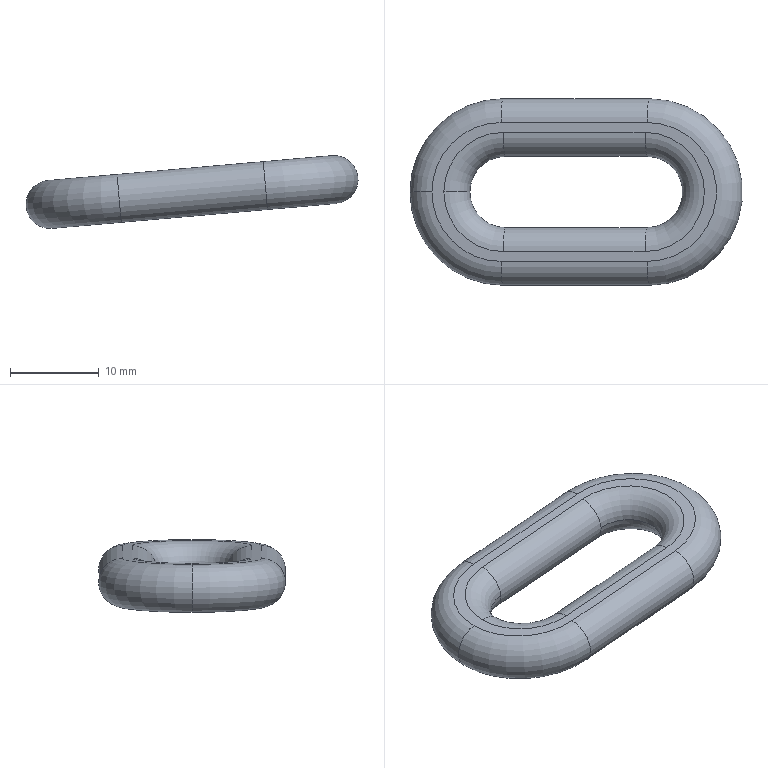Part | STEP file | 871-10_1m (label)-Part-1 | 1 solid | 15 faces | box 37.378 x 21 x 8.198 mm | volume 2290 mm3 | torus 9 | cylinder 4 | plane 2 | commonest cylinder face diameters 5.4 x4
STEP:
#1=CARTESIAN_POINT('',(0.,0.,0.));
#2=DIRECTION('',(0.,0.,1.));
#3=DIRECTION('',(1.,0.,0.));
#4=AXIS2_PLACEMENT_3D('',#1,#2,#3);
#5=CARTESIAN_POINT('',(26.368,17.2,8.756));
#6=VERTEX_POINT('',#5);
#7=CARTESIAN_POINT('',(26.603,14.5,6.066));
#8=VERTEX_POINT('',#7);
#9=CARTESIAN_POINT('',(26.603,17.2,6.066));
#10=DIRECTION('',(0.9962,0.,0.08716));
#11=DIRECTION('',(0.08716,0.,-0.9962));
#12=AXIS2_PLACEMENT_3D('',#9,#10,#11);
#13=CIRCLE('',#12,2.7);
#14=CARTESIAN_POINT('',(26.603,10.5,6.066));
#15=DIRECTION('',(0.08716,0.,-0.9962));
#16=DIRECTION('',(-0.9962,0.,-0.08716));
#17=AXIS2_PLACEMENT_3D('',#14,#15,#16);
#18=TOROIDAL_SURFACE('',#17,6.7,2.7);
#19=CARTESIAN_POINT('',(1.571,7.854));
#20=DIRECTION('',(0.,-1.));
#21=VECTOR('',#20,1.);
#22=LINE('',#19,#21);
#23=(GEOMETRIC_REPRESENTATION_CONTEXT(2)PARAMETRIC_REPRESENTATION_CONTEXT()REPRESENTATION_CONTEXT('',''));
#24=DEFINITIONAL_REPRESENTATION('',(#22),#23);
#25=PCURVE('',#18,#24);
#26=CARTESIAN_POINT('',(18.633,17.2,5.369));
#27=DIRECTION('',(0.9962,0.,0.08716));
#28=DIRECTION('',(0.08716,0.,-0.9962));
#29=AXIS2_PLACEMENT_3D('',#26,#27,#28);
#30=CYLINDRICAL_SURFACE('',#29,2.7);
#31=CARTESIAN_POINT('',(0.,8.));
#32=DIRECTION('',(1.,0.));
#33=VECTOR('',#32,1.);
#34=LINE('',#31,#33);
#35=(GEOMETRIC_REPRESENTATION_CONTEXT(2)PARAMETRIC_REPRESENTATION_CONTEXT()REPRESENTATION_CONTEXT('',''));
#36=DEFINITIONAL_REPRESENTATION('',(#34),#35);
#37=PCURVE('',#30,#36);
#38=SURFACE_CURVE('',#13,(#25,#37),.PCURVE_S1.);
#39=EDGE_CURVE('',#6,#8,#38,.T.);
#40=ORIENTED_EDGE('',*,*,#39,.T.);
#41=CARTESIAN_POINT('',(26.603,6.5,6.066));
#42=VERTEX_POINT('',#41);
#43=CARTESIAN_POINT('',(26.603,10.5,6.066));
#44=DIRECTION('',(0.08716,0.,-0.9962));
#45=DIRECTION('',(-0.9962,0.,-0.08716));
#46=AXIS2_PLACEMENT_3D('',#43,#44,#45);
#47=CIRCLE('',#46,4.);
#48=CARTESIAN_POINT('',(0.,3.142));
#49=DIRECTION('',(1.,0.));
#50=VECTOR('',#49,1.);
#51=LINE('',#48,#50);
#52=(GEOMETRIC_REPRESENTATION_CONTEXT(2)PARAMETRIC_REPRESENTATION_CONTEXT()REPRESENTATION_CONTEXT('',''));
#53=DEFINITIONAL_REPRESENTATION('',(#51),#52);
#54=PCURVE('',#18,#53);
#55=CARTESIAN_POINT('',(26.603,10.5,6.066));
#56=DIRECTION('',(0.08716,0.,-0.9962));
#57=DIRECTION('',(-0.9962,0.,-0.08716));
#58=AXIS2_PLACEMENT_3D('',#55,#56,#57);
#59=TOROIDAL_SURFACE('',#58,6.7,2.7);
#60=CARTESIAN_POINT('',(0.,3.142));
#61=DIRECTION('',(1.,0.));
#62=VECTOR('',#61,1.);
#63=LINE('',#60,#62);
#64=(GEOMETRIC_REPRESENTATION_CONTEXT(2)PARAMETRIC_REPRESENTATION_CONTEXT()REPRESENTATION_CONTEXT('',''));
#65=DEFINITIONAL_REPRESENTATION('',(#63),#64);
#66=PCURVE('',#59,#65);
#67=SURFACE_CURVE('',#47,(#54,#66),.PCURVE_S1.);
#68=EDGE_CURVE('',#8,#42,#67,.T.);
#69=ORIENTED_EDGE('',*,*,#68,.T.);
#70=CARTESIAN_POINT('',(26.368,3.8,8.756));
#71=VERTEX_POINT('',#70);
#72=CARTESIAN_POINT('',(26.603,3.8,6.066));
#73=DIRECTION('',(-0.9962,0.,-0.08716));
#74=DIRECTION('',(-0.08716,0.,0.9962));
#75=AXIS2_PLACEMENT_3D('',#72,#73,#74);
#76=CIRCLE('',#75,2.7);
#77=CARTESIAN_POINT('',(4.712,4.712));
#78=DIRECTION('',(0.,-1.));
#79=VECTOR('',#78,1.);
#80=LINE('',#77,#79);
#81=(GEOMETRIC_REPRESENTATION_CONTEXT(2)PARAMETRIC_REPRESENTATION_CONTEXT()REPRESENTATION_CONTEXT('',''));
#82=DEFINITIONAL_REPRESENTATION('',(#80),#81);
#83=PCURVE('',#18,#82);
#84=CARTESIAN_POINT('',(18.633,3.8,5.369));
#85=DIRECTION('',(-0.9962,0.,-0.08716));
#86=DIRECTION('',(-0.08716,0.,0.9962));
#87=AXIS2_PLACEMENT_3D('',#84,#85,#86);
#88=CYLINDRICAL_SURFACE('',#87,2.7);
#89=CARTESIAN_POINT('',(0.,-8.));
#90=DIRECTION('',(1.,0.));
#91=VECTOR('',#90,1.);
#92=LINE('',#89,#91);
#93=(GEOMETRIC_REPRESENTATION_CONTEXT(2)PARAMETRIC_REPRESENTATION_CONTEXT()REPRESENTATION_CONTEXT('',''));
#94=DEFINITIONAL_REPRESENTATION('',(#92),#93);
#95=PCURVE('',#88,#94);
#96=SURFACE_CURVE('',#76,(#83,#95),.PCURVE_S1.);
#97=EDGE_CURVE('',#71,#42,#96,.T.);
#98=ORIENTED_EDGE('',*,*,#97,.F.);
#99=CARTESIAN_POINT('',(26.368,10.5,8.756));
#100=DIRECTION('',(0.08716,0.,-0.9962));
#101=DIRECTION('',(0.9962,0.,0.08716));
#102=AXIS2_PLACEMENT_3D('',#99,#100,#101);
#103=CIRCLE('',#102,6.7);
#104=CARTESIAN_POINT('',(-3.142,4.712));
#105=DIRECTION('',(1.,0.));
#106=VECTOR('',#105,1.);
#107=LINE('',#104,#106);
#108=(GEOMETRIC_REPRESENTATION_CONTEXT(2)PARAMETRIC_REPRESENTATION_CONTEXT()REPRESENTATION_CONTEXT('',''));
#109=DEFINITIONAL_REPRESENTATION('',(#107),#108);
#110=PCURVE('',#18,#109);
#111=CARTESIAN_POINT('',(18.398,10.5,8.059));
#112=DIRECTION('',(-0.08716,0.,0.9962));
#113=DIRECTION('',(0.9962,0.,0.08716));
#114=AXIS2_PLACEMENT_3D('',#111,#112,#113);
#115=PLANE('',#114);
#116=CARTESIAN_POINT('',(14.7,0.));
#117=CARTESIAN_POINT('',(14.7,-11.605));
#118=CARTESIAN_POINT('',(4.65,-5.802));
#119=CARTESIAN_POINT('',(-5.4,0.));
#120=CARTESIAN_POINT('',(4.65,5.802));
#121=CARTESIAN_POINT('',(14.7,11.605));
#122=CARTESIAN_POINT('',(14.7,0.));
#123=(BOUNDED_CURVE()B_SPLINE_CURVE(2,(#116,#117,#118,#119,#120,#121,#122),.UNSPECIFIED.,.T.,.F.)B_SPLINE_CURVE_WITH_KNOTS((1,2,2,2,2,1),(-2.094,0.,2.094,4.189,6.283,8.378),.UNSPECIFIED.)CURVE()GEOMETRIC_REPRESENTATION_ITEM()RATIONAL_B_SPLINE_CURVE((1.,0.5,1.,0.5,1.,0.5,1.))REPRESENTATION_ITEM(''));
#124=(GEOMETRIC_REPRESENTATION_CONTEXT(2)PARAMETRIC_REPRESENTATION_CONTEXT()REPRESENTATION_CONTEXT('',''));
#125=DEFINITIONAL_REPRESENTATION('',(#123),#124);
#126=PCURVE('',#115,#125);
#127=SURFACE_CURVE('',#103,(#110,#126),.PCURVE_S1.);
#128=EDGE_CURVE('',#6,#71,#127,.T.);
#129=ORIENTED_EDGE('',*,*,#128,.F.);
#130=EDGE_LOOP('',(#40,#69,#98,#129));
#131=FACE_BOUND('',#130,.T.);
#132=ADVANCED_FACE('',(#131),#18,.T.);
#133=CARTESIAN_POINT('',(6.679,10.5,4.323));
#134=VERTEX_POINT('',#133);
#135=CARTESIAN_POINT('',(3.754,10.5,6.778));
#136=VERTEX_POINT('',#135);
#137=CARTESIAN_POINT('',(3.989,10.5,4.088));
#138=DIRECTION('',(0.,-1.,0.));
#139=DIRECTION('',(1.,0.,0.));
#140=AXIS2_PLACEMENT_3D('',#137,#138,#139);
#141=CIRCLE('',#140,2.7);
#142=CARTESIAN_POINT('',(10.664,10.5,4.672));
#143=DIRECTION('',(0.08716,0.,-0.9962));
#144=DIRECTION('',(-0.9962,0.,-0.08716));
#145=AXIS2_PLACEMENT_3D('',#142,#143,#144);
#146=TOROIDAL_SURFACE('',#145,6.7,2.7);
#147=CARTESIAN_POINT('',(0.,3.054));
#148=DIRECTION('',(0.,1.));
#149=VECTOR('',#148,1.);
#150=LINE('',#147,#149);
#151=(GEOMETRIC_REPRESENTATION_CONTEXT(2)PARAMETRIC_REPRESENTATION_CONTEXT()REPRESENTATION_CONTEXT('',''));
#152=DEFINITIONAL_REPRESENTATION('',(#150),#151);
#153=PCURVE('',#146,#152);
#154=CARTESIAN_POINT('',(10.664,10.5,4.672));
#155=DIRECTION('',(0.08716,0.,-0.9962));
#156=DIRECTION('',(-0.9962,0.,-0.08716));
#157=AXIS2_PLACEMENT_3D('',#154,#155,#156);
#158=TOROIDAL_SURFACE('',#157,6.7,2.7);
#159=CARTESIAN_POINT('',(6.283,3.054));
#160=DIRECTION('',(0.,1.));
#161=VECTOR('',#160,1.);
#162=LINE('',#159,#161);
#163=(GEOMETRIC_REPRESENTATION_CONTEXT(2)PARAMETRIC_REPRESENTATION_CONTEXT()REPRESENTATION_CONTEXT('',''));
#164=DEFINITIONAL_REPRESENTATION('',(#162),#163);
#165=PCURVE('',#158,#164);
#166=SURFACE_CURVE('',#141,(#153,#165),.PCURVE_S1.);
#167=EDGE_CURVE('',#134,#136,#166,.T.);
#168=ORIENTED_EDGE('',*,*,#167,.F.);
#169=CARTESIAN_POINT('',(10.664,14.5,4.672));
#170=VERTEX_POINT('',#169);
#171=CARTESIAN_POINT('',(10.664,10.5,4.672));
#172=DIRECTION('',(0.08716,0.,-0.9962));
#173=DIRECTION('',(-0.9962,0.,-0.08716));
#174=AXIS2_PLACEMENT_3D('',#171,#172,#173);
#175=CIRCLE('',#174,4.);
#176=CARTESIAN_POINT('',(0.,3.142));
#177=DIRECTION('',(1.,0.));
#178=VECTOR('',#177,1.);
#179=LINE('',#176,#178);
#180=(GEOMETRIC_REPRESENTATION_CONTEXT(2)PARAMETRIC_REPRESENTATION_CONTEXT()REPRESENTATION_CONTEXT('',''));
#181=DEFINITIONAL_REPRESENTATION('',(#179),#180);
#182=PCURVE('',#146,#181);
#183=CARTESIAN_POINT('',(10.664,10.5,4.672));
#184=DIRECTION('',(0.08716,0.,-0.9962));
#185=DIRECTION('',(-0.9962,0.,-0.08716));
#186=AXIS2_PLACEMENT_3D('',#183,#184,#185);
#187=TOROIDAL_SURFACE('',#186,6.7,2.7);
#188=CARTESIAN_POINT('',(0.,3.142));
#189=DIRECTION('',(1.,0.));
#190=VECTOR('',#189,1.);
#191=LINE('',#188,#190);
#192=(GEOMETRIC_REPRESENTATION_CONTEXT(2)PARAMETRIC_REPRESENTATION_CONTEXT()REPRESENTATION_CONTEXT('',''));
#193=DEFINITIONAL_REPRESENTATION('',(#191),#192);
#194=PCURVE('',#187,#193);
#195=SURFACE_CURVE('',#175,(#182,#194),.PCURVE_S1.);
#196=EDGE_CURVE('',#134,#170,#195,.T.);
#197=ORIENTED_EDGE('',*,*,#196,.T.);
#198=CARTESIAN_POINT('',(10.429,17.2,7.362));
#199=VERTEX_POINT('',#198);
#200=CARTESIAN_POINT('',(10.664,17.2,4.672));
#201=DIRECTION('',(-0.9962,0.,-0.08716));
#202=DIRECTION('',(-0.08716,0.,0.9962));
#203=AXIS2_PLACEMENT_3D('',#200,#201,#202);
#204=CIRCLE('',#203,2.7);
#205=CARTESIAN_POINT('',(1.571,-1.571));
#206=DIRECTION('',(0.,1.));
#207=VECTOR('',#206,1.);
#208=LINE('',#205,#207);
#209=(GEOMETRIC_REPRESENTATION_CONTEXT(2)PARAMETRIC_REPRESENTATION_CONTEXT()REPRESENTATION_CONTEXT('',''));
#210=DEFINITIONAL_REPRESENTATION('',(#208),#209);
#211=PCURVE('',#146,#210);
#212=CARTESIAN_POINT('',(9.425,-8.));
#213=DIRECTION('',(-1.,0.));
#214=VECTOR('',#213,1.);
#215=LINE('',#212,#214);
#216=(GEOMETRIC_REPRESENTATION_CONTEXT(2)PARAMETRIC_REPRESENTATION_CONTEXT()REPRESENTATION_CONTEXT('',''));
#217=DEFINITIONAL_REPRESENTATION('',(#215),#216);
#218=PCURVE('',#30,#217);
#219=SURFACE_CURVE('',#204,(#211,#218),.PCURVE_S1.);
#220=EDGE_CURVE('',#170,#199,#219,.T.);
#221=ORIENTED_EDGE('',*,*,#220,.T.);
#222=CARTESIAN_POINT('',(10.429,10.5,7.362));
#223=DIRECTION('',(0.08716,0.,-0.9962));
#224=DIRECTION('',(0.9962,0.,0.08716));
#225=AXIS2_PLACEMENT_3D('',#222,#223,#224);
#226=CIRCLE('',#225,6.7);
#227=CARTESIAN_POINT('',(-3.142,4.712));
#228=DIRECTION('',(1.,0.));
#229=VECTOR('',#228,1.);
#230=LINE('',#227,#229);
#231=(GEOMETRIC_REPRESENTATION_CONTEXT(2)PARAMETRIC_REPRESENTATION_CONTEXT()REPRESENTATION_CONTEXT('',''));
#232=DEFINITIONAL_REPRESENTATION('',(#230),#231);
#233=PCURVE('',#146,#232);
#234=CARTESIAN_POINT('',(-1.3,0.));
#235=CARTESIAN_POINT('',(-1.3,-11.605));
#236=CARTESIAN_POINT('',(-11.35,-5.802));
#237=CARTESIAN_POINT('',(-21.4,0.));
#238=CARTESIAN_POINT('',(-11.35,5.802));
#239=CARTESIAN_POINT('',(-1.3,11.605));
#240=CARTESIAN_POINT('',(-1.3,0.));
#241=(BOUNDED_CURVE()B_SPLINE_CURVE(2,(#234,#235,#236,#237,#238,#239,#240),.UNSPECIFIED.,.T.,.F.)B_SPLINE_CURVE_WITH_KNOTS((1,2,2,2,2,1),(-2.094,0.,2.094,4.189,6.283,8.378),.UNSPECIFIED.)CURVE()GEOMETRIC_REPRESENTATION_ITEM()RATIONAL_B_SPLINE_CURVE((1.,0.5,1.,0.5,1.,0.5,1.))REPRESENTATION_ITEM(''));
#242=(GEOMETRIC_REPRESENTATION_CONTEXT(2)PARAMETRIC_REPRESENTATION_CONTEXT()REPRESENTATION_CONTEXT('',''));
#243=DEFINITIONAL_REPRESENTATION('',(#241),#242);
#244=PCURVE('',#115,#243);
#245=SURFACE_CURVE('',#226,(#233,#244),.PCURVE_S1.);
#246=EDGE_CURVE('',#136,#199,#245,.T.);
#247=ORIENTED_EDGE('',*,*,#246,.F.);
#248=EDGE_LOOP('',(#168,#197,#221,#247));
#249=FACE_BOUND('',#248,.T.);
#250=ADVANCED_FACE('',(#249),#146,.T.);
#251=CARTESIAN_POINT('',(10.664,6.5,4.672));
#252=VERTEX_POINT('',#251);
#253=CARTESIAN_POINT('',(10.429,3.8,7.362));
#254=VERTEX_POINT('',#253);
#255=CARTESIAN_POINT('',(10.664,3.8,4.672));
#256=DIRECTION('',(0.9962,0.,0.08716));
#257=DIRECTION('',(0.08716,0.,-0.9962));
#258=AXIS2_PLACEMENT_3D('',#255,#256,#257);
#259=CIRCLE('',#258,2.7);
#260=CARTESIAN_POINT('',(4.712,1.571));
#261=DIRECTION('',(0.,1.));
#262=VECTOR('',#261,1.);
#263=LINE('',#260,#262);
#264=(GEOMETRIC_REPRESENTATION_CONTEXT(2)PARAMETRIC_REPRESENTATION_CONTEXT()REPRESENTATION_CONTEXT('',''));
#265=DEFINITIONAL_REPRESENTATION('',(#263),#264);
#266=PCURVE('',#158,#265);
#267=CARTESIAN_POINT('',(3.142,8.));
#268=DIRECTION('',(-1.,0.));
#269=VECTOR('',#268,1.);
#270=LINE('',#267,#269);
#271=(GEOMETRIC_REPRESENTATION_CONTEXT(2)PARAMETRIC_REPRESENTATION_CONTEXT()REPRESENTATION_CONTEXT('',''));
#272=DEFINITIONAL_REPRESENTATION('',(#270),#271);
#273=PCURVE('',#88,#272);
#274=SURFACE_CURVE('',#259,(#266,#273),.PCURVE_S1.);
#275=EDGE_CURVE('',#252,#254,#274,.T.);
#276=ORIENTED_EDGE('',*,*,#275,.F.);
#277=CARTESIAN_POINT('',(10.664,10.5,4.672));
#278=DIRECTION('',(0.08716,0.,-0.9962));
#279=DIRECTION('',(-0.9962,0.,-0.08716));
#280=AXIS2_PLACEMENT_3D('',#277,#278,#279);
#281=CIRCLE('',#280,4.);
#282=CARTESIAN_POINT('',(0.,3.142));
#283=DIRECTION('',(1.,0.));
#284=VECTOR('',#283,1.);
#285=LINE('',#282,#284);
#286=(GEOMETRIC_REPRESENTATION_CONTEXT(2)PARAMETRIC_REPRESENTATION_CONTEXT()REPRESENTATION_CONTEXT('',''));
#287=DEFINITIONAL_REPRESENTATION('',(#285),#286);
#288=PCURVE('',#158,#287);
#289=CARTESIAN_POINT('',(10.664,10.5,4.672));
#290=DIRECTION('',(0.08716,0.,-0.9962));
#291=DIRECTION('',(-0.9962,0.,-0.08716));
#292=AXIS2_PLACEMENT_3D('',#289,#290,#291);
#293=TOROIDAL_SURFACE('',#292,6.7,2.7);
#294=CARTESIAN_POINT('',(0.,3.142));
#295=DIRECTION('',(1.,0.));
#296=VECTOR('',#295,1.);
#297=LINE('',#294,#296);
#298=(GEOMETRIC_REPRESENTATION_CONTEXT(2)PARAMETRIC_REPRESENTATION_CONTEXT()REPRESENTATION_CONTEXT('',''));
#299=DEFINITIONAL_REPRESENTATION('',(#297),#298);
#300=PCURVE('',#293,#299);
#301=SURFACE_CURVE('',#281,(#288,#300),.PCURVE_S1.);
#302=EDGE_CURVE('',#252,#134,#301,.T.);
#303=ORIENTED_EDGE('',*,*,#302,.T.);
#304=ORIENTED_EDGE('',*,*,#167,.T.);
#305=CARTESIAN_POINT('',(10.429,10.5,7.362));
#306=DIRECTION('',(0.08716,0.,-0.9962));
#307=DIRECTION('',(0.9962,0.,0.08716));
#308=AXIS2_PLACEMENT_3D('',#305,#306,#307);
#309=CIRCLE('',#308,6.7);
#310=CARTESIAN_POINT('',(3.142,4.712));
#311=DIRECTION('',(1.,0.));
#312=VECTOR('',#311,1.);
#313=LINE('',#310,#312);
#314=(GEOMETRIC_REPRESENTATION_CONTEXT(2)PARAMETRIC_REPRESENTATION_CONTEXT()REPRESENTATION_CONTEXT('',''));
#315=DEFINITIONAL_REPRESENTATION('',(#313),#314);
#316=PCURVE('',#158,#315);
#317=CARTESIAN_POINT('',(-1.3,0.));
#318=CARTESIAN_POINT('',(-1.3,-11.605));
#319=CARTESIAN_POINT('',(-11.35,-5.802));
#320=CARTESIAN_POINT('',(-21.4,0.));
#321=CARTESIAN_POINT('',(-11.35,5.802));
#322=CARTESIAN_POINT('',(-1.3,11.605));
#323=CARTESIAN_POINT('',(-1.3,0.));
#324=(BOUNDED_CURVE()B_SPLINE_CURVE(2,(#317,#318,#319,#320,#321,#322,#323),.UNSPECIFIED.,.T.,.F.)B_SPLINE_CURVE_WITH_KNOTS((1,2,2,2,2,1),(-2.094,0.,2.094,4.189,6.283,8.378),.UNSPECIFIED.)CURVE()GEOMETRIC_REPRESENTATION_ITEM()RATIONAL_B_SPLINE_CURVE((1.,0.5,1.,0.5,1.,0.5,1.))REPRESENTATION_ITEM(''));
#325=(GEOMETRIC_REPRESENTATION_CONTEXT(2)PARAMETRIC_REPRESENTATION_CONTEXT()REPRESENTATION_CONTEXT('',''));
#326=DEFINITIONAL_REPRESENTATION('',(#324),#325);
#327=PCURVE('',#115,#326);
#328=SURFACE_CURVE('',#309,(#316,#327),.PCURVE_S1.);
#329=EDGE_CURVE('',#254,#136,#328,.T.);
#330=ORIENTED_EDGE('',*,*,#329,.F.);
#331=EDGE_LOOP('',(#276,#303,#304,#330));
#332=FACE_BOUND('',#331,.T.);
#333=ADVANCED_FACE('',(#332),#158,.T.);
#334=ORIENTED_EDGE('',*,*,#302,.F.);
#335=CARTESIAN_POINT('',(10.899,3.8,1.982));
#336=VERTEX_POINT('',#335);
#337=CARTESIAN_POINT('',(10.664,3.8,4.672));
#338=DIRECTION('',(0.9962,0.,0.08716));
#339=DIRECTION('',(0.08716,0.,-0.9962));
#340=AXIS2_PLACEMENT_3D('',#337,#338,#339);
#341=CIRCLE('',#340,2.7);
#342=CARTESIAN_POINT('',(4.712,1.571));
#343=DIRECTION('',(0.,1.));
#344=VECTOR('',#343,1.);
#345=LINE('',#342,#344);
#346=(GEOMETRIC_REPRESENTATION_CONTEXT(2)PARAMETRIC_REPRESENTATION_CONTEXT()REPRESENTATION_CONTEXT('',''));
#347=DEFINITIONAL_REPRESENTATION('',(#345),#346);
#348=PCURVE('',#293,#347);
#349=CARTESIAN_POINT('',(3.142,8.));
#350=DIRECTION('',(-1.,0.));
#351=VECTOR('',#350,1.);
#352=LINE('',#349,#351);
#353=(GEOMETRIC_REPRESENTATION_CONTEXT(2)PARAMETRIC_REPRESENTATION_CONTEXT()REPRESENTATION_CONTEXT('',''));
#354=DEFINITIONAL_REPRESENTATION('',(#352),#353);
#355=PCURVE('',#88,#354);
#356=SURFACE_CURVE('',#341,(#348,#355),.PCURVE_S1.);
#357=EDGE_CURVE('',#336,#252,#356,.T.);
#358=ORIENTED_EDGE('',*,*,#357,.F.);
#359=CARTESIAN_POINT('',(4.225,10.5,1.398));
#360=VERTEX_POINT('',#359);
#361=CARTESIAN_POINT('',(10.899,10.5,1.982));
#362=DIRECTION('',(-0.08716,0.,0.9962));
#363=DIRECTION('',(-0.9962,0.,-0.08716));
#364=AXIS2_PLACEMENT_3D('',#361,#362,#363);
#365=CIRCLE('',#364,6.7);
#366=CARTESIAN_POINT('',(6.283,1.571));
#367=DIRECTION('',(-1.,0.));
#368=VECTOR('',#367,1.);
#369=LINE('',#366,#368);
#370=(GEOMETRIC_REPRESENTATION_CONTEXT(2)PARAMETRIC_REPRESENTATION_CONTEXT()REPRESENTATION_CONTEXT('',''));
#371=DEFINITIONAL_REPRESENTATION('',(#369),#370);
#372=PCURVE('',#293,#371);
#373=CARTESIAN_POINT('',(18.869,10.5,2.679));
#374=DIRECTION('',(0.08716,0.,-0.9962));
#375=DIRECTION('',(-0.9962,0.,-0.08716));
#376=AXIS2_PLACEMENT_3D('',#373,#374,#375);
#377=PLANE('',#376);
#378=CARTESIAN_POINT('',(14.7,0.));
#379=CARTESIAN_POINT('',(14.7,-11.605));
#380=CARTESIAN_POINT('',(4.65,-5.802));
#381=CARTESIAN_POINT('',(-5.4,0.));
#382=CARTESIAN_POINT('',(4.65,5.802));
#383=CARTESIAN_POINT('',(14.7,11.605));
#384=CARTESIAN_POINT('',(14.7,0.));
#385=(BOUNDED_CURVE()B_SPLINE_CURVE(2,(#378,#379,#380,#381,#382,#383,#384),.UNSPECIFIED.,.T.,.F.)B_SPLINE_CURVE_WITH_KNOTS((1,2,2,2,2,1),(-2.094,0.,2.094,4.189,6.283,8.378),.UNSPECIFIED.)CURVE()GEOMETRIC_REPRESENTATION_ITEM()RATIONAL_B_SPLINE_CURVE((1.,0.5,1.,0.5,1.,0.5,1.))REPRESENTATION_ITEM(''));
#386=(GEOMETRIC_REPRESENTATION_CONTEXT(2)PARAMETRIC_REPRESENTATION_CONTEXT()REPRESENTATION_CONTEXT('',''));
#387=DEFINITIONAL_REPRESENTATION('',(#385),#386);
#388=PCURVE('',#377,#387);
#389=SURFACE_CURVE('',#365,(#372,#388),.PCURVE_S1.);
#390=EDGE_CURVE('',#360,#336,#389,.T.);
#391=ORIENTED_EDGE('',*,*,#390,.F.);
#392=CARTESIAN_POINT('',(3.989,10.5,4.088));
#393=DIRECTION('',(0.,-1.,0.));
#394=DIRECTION('',(1.,0.,0.));
#395=AXIS2_PLACEMENT_3D('',#392,#393,#394);
#396=CIRCLE('',#395,2.7);
#397=CARTESIAN_POINT('',(6.283,-3.229));
#398=DIRECTION('',(0.,1.));
#399=VECTOR('',#398,1.);
#400=LINE('',#397,#399);
#401=(GEOMETRIC_REPRESENTATION_CONTEXT(2)PARAMETRIC_REPRESENTATION_CONTEXT()REPRESENTATION_CONTEXT('',''));
#402=DEFINITIONAL_REPRESENTATION('',(#400),#401);
#403=PCURVE('',#293,#402);
#404=CARTESIAN_POINT('',(0.,-3.229));
#405=DIRECTION('',(0.,1.));
#406=VECTOR('',#405,1.);
#407=LINE('',#404,#406);
#408=(GEOMETRIC_REPRESENTATION_CONTEXT(2)PARAMETRIC_REPRESENTATION_CONTEXT()REPRESENTATION_CONTEXT('',''));
#409=DEFINITIONAL_REPRESENTATION('',(#407),#408);
#410=PCURVE('',#187,#409);
#411=SURFACE_CURVE('',#396,(#403,#410),.PCURVE_S1.);
#412=EDGE_CURVE('',#360,#134,#411,.T.);
#413=ORIENTED_EDGE('',*,*,#412,.T.);
#414=EDGE_LOOP('',(#334,#358,#391,#413));
#415=FACE_BOUND('',#414,.T.);
#416=ADVANCED_FACE('',(#415),#293,.T.);
#417=CARTESIAN_POINT('',(2.409,10.5,6.66));
#418=VERTEX_POINT('',#417);
#419=CARTESIAN_POINT('',(10.18,2.7,7.34));
#420=VERTEX_POINT('',#419);
#421=CARTESIAN_POINT('',(10.18,10.5,7.34));
#422=DIRECTION('',(-0.08716,0.,0.9962));
#423=DIRECTION('',(0.9962,0.,0.08716));
#424=AXIS2_PLACEMENT_3D('',#421,#422,#423);
#425=CIRCLE('',#424,7.8);
#426=CARTESIAN_POINT('',(10.415,10.5,4.65));
#427=DIRECTION('',(0.08716,0.,-0.9962));
#428=DIRECTION('',(-0.9962,0.,-0.08716));
#429=AXIS2_PLACEMENT_3D('',#426,#427,#428);
#430=TOROIDAL_SURFACE('',#429,7.8,2.7);
#431=CARTESIAN_POINT('',(9.425,-1.571));
#432=DIRECTION('',(-1.,0.));
#433=VECTOR('',#432,1.);
#434=LINE('',#431,#433);
#435=(GEOMETRIC_REPRESENTATION_CONTEXT(2)PARAMETRIC_REPRESENTATION_CONTEXT()REPRESENTATION_CONTEXT('',''));
#436=DEFINITIONAL_REPRESENTATION('',(#434),#435);
#437=PCURVE('',#430,#436);
#438=CARTESIAN_POINT('',(-8.25,0.));
#439=DIRECTION('',(1.,0.));
#440=AXIS2_PLACEMENT_2D('',#438,#439);
#441=CIRCLE('',#440,7.8);
#442=(GEOMETRIC_REPRESENTATION_CONTEXT(2)PARAMETRIC_REPRESENTATION_CONTEXT()REPRESENTATION_CONTEXT('',''));
#443=DEFINITIONAL_REPRESENTATION('',(#441),#442);
#444=PCURVE('',#115,#443);
#445=SURFACE_CURVE('',#425,(#437,#444),.PCURVE_S1.);
#446=EDGE_CURVE('',#418,#420,#445,.T.);
#447=ORIENTED_EDGE('',*,*,#446,.F.);
#448=CARTESIAN_POINT('',(2.88,10.5,1.281));
#449=VERTEX_POINT('',#448);
#450=CARTESIAN_POINT('',(2.645,10.5,3.97));
#451=DIRECTION('',(0.,-1.,0.));
#452=DIRECTION('',(1.,0.,0.));
#453=AXIS2_PLACEMENT_3D('',#450,#451,#452);
#454=CIRCLE('',#453,2.7);
#455=CARTESIAN_POINT('',(6.283,-3.229));
#456=DIRECTION('',(0.,1.));
#457=VECTOR('',#456,1.);
#458=LINE('',#455,#457);
#459=(GEOMETRIC_REPRESENTATION_CONTEXT(2)PARAMETRIC_REPRESENTATION_CONTEXT()REPRESENTATION_CONTEXT('',''));
#460=DEFINITIONAL_REPRESENTATION('',(#458),#459);
#461=PCURVE('',#430,#460);
#462=CARTESIAN_POINT('',(10.415,10.5,4.65));
#463=DIRECTION('',(0.08716,0.,-0.9962));
#464=DIRECTION('',(-0.9962,0.,-0.08716));
#465=AXIS2_PLACEMENT_3D('',#462,#463,#464);
#466=TOROIDAL_SURFACE('',#465,7.8,2.7);
#467=CARTESIAN_POINT('',(0.,3.054));
#468=DIRECTION('',(0.,1.));
#469=VECTOR('',#468,1.);
#470=LINE('',#467,#469);
#471=(GEOMETRIC_REPRESENTATION_CONTEXT(2)PARAMETRIC_REPRESENTATION_CONTEXT()REPRESENTATION_CONTEXT('',''));
#472=DEFINITIONAL_REPRESENTATION('',(#470),#471);
#473=PCURVE('',#466,#472);
#474=SURFACE_CURVE('',#454,(#461,#473),.PCURVE_S1.);
#475=EDGE_CURVE('',#418,#449,#474,.T.);
#476=ORIENTED_EDGE('',*,*,#475,.T.);
#477=CARTESIAN_POINT('',(10.65,2.7,1.96));
#478=VERTEX_POINT('',#477);
#479=CARTESIAN_POINT('',(10.65,10.5,1.96));
#480=DIRECTION('',(0.08716,0.,-0.9962));
#481=DIRECTION('',(-0.9962,0.,-0.08716));
#482=AXIS2_PLACEMENT_3D('',#479,#480,#481);
#483=CIRCLE('',#482,7.8);
#484=CARTESIAN_POINT('',(0.,1.571));
#485=DIRECTION('',(1.,0.));
#486=VECTOR('',#485,1.);
#487=LINE('',#484,#486);
#488=(GEOMETRIC_REPRESENTATION_CONTEXT(2)PARAMETRIC_REPRESENTATION_CONTEXT()REPRESENTATION_CONTEXT('',''));
#489=DEFINITIONAL_REPRESENTATION('',(#487),#488);
#490=PCURVE('',#430,#489);
#491=CARTESIAN_POINT('',(8.25,0.));
#492=DIRECTION('',(1.,0.));
#493=AXIS2_PLACEMENT_2D('',#491,#492);
#494=CIRCLE('',#493,7.8);
#495=(GEOMETRIC_REPRESENTATION_CONTEXT(2)PARAMETRIC_REPRESENTATION_CONTEXT()REPRESENTATION_CONTEXT('',''));
#496=DEFINITIONAL_REPRESENTATION('',(#494),#495);
#497=PCURVE('',#377,#496);
#498=SURFACE_CURVE('',#483,(#490,#497),.PCURVE_S1.);
#499=EDGE_CURVE('',#478,#449,#498,.T.);
#500=ORIENTED_EDGE('',*,*,#499,.F.);
#501=CARTESIAN_POINT('',(10.415,2.7,4.65));
#502=DIRECTION('',(0.9962,0.,0.08716));
#503=DIRECTION('',(0.08716,0.,-0.9962));
#504=AXIS2_PLACEMENT_3D('',#501,#502,#503);
#505=CIRCLE('',#504,2.7);
#506=CARTESIAN_POINT('',(4.712,-4.712));
#507=DIRECTION('',(0.,1.));
#508=VECTOR('',#507,1.);
#509=LINE('',#506,#508);
#510=(GEOMETRIC_REPRESENTATION_CONTEXT(2)PARAMETRIC_REPRESENTATION_CONTEXT()REPRESENTATION_CONTEXT('',''));
#511=DEFINITIONAL_REPRESENTATION('',(#509),#510);
#512=PCURVE('',#430,#511);
#513=CARTESIAN_POINT('',(18.633,2.7,5.369));
#514=DIRECTION('',(0.9962,0.,0.08716));
#515=DIRECTION('',(0.08716,0.,-0.9962));
#516=AXIS2_PLACEMENT_3D('',#513,#514,#515);
#517=CYLINDRICAL_SURFACE('',#516,2.7);
#518=CARTESIAN_POINT('',(0.,-8.25));
#519=DIRECTION('',(1.,0.));
#520=VECTOR('',#519,1.);
#521=LINE('',#518,#520);
#522=(GEOMETRIC_REPRESENTATION_CONTEXT(2)PARAMETRIC_REPRESENTATION_CONTEXT()REPRESENTATION_CONTEXT('',''));
#523=DEFINITIONAL_REPRESENTATION('',(#521),#522);
#524=PCURVE('',#517,#523);
#525=SURFACE_CURVE('',#505,(#512,#524),.PCURVE_S1.);
#526=EDGE_CURVE('',#420,#478,#525,.T.);
#527=ORIENTED_EDGE('',*,*,#526,.F.);
#528=EDGE_LOOP('',(#447,#476,#500,#527));
#529=FACE_BOUND('',#528,.T.);
#530=ADVANCED_FACE('',(#529),#430,.T.);
#531=CARTESIAN_POINT('',(10.899,17.2,1.982));
#532=VERTEX_POINT('',#531);
#533=CARTESIAN_POINT('',(10.899,10.5,1.982));
#534=DIRECTION('',(-0.08716,0.,0.9962));
#535=DIRECTION('',(-0.9962,0.,-0.08716));
#536=AXIS2_PLACEMENT_3D('',#533,#534,#535);
#537=CIRCLE('',#536,6.7);
#538=CARTESIAN_POINT('',(14.7,0.));
#539=CARTESIAN_POINT('',(14.7,-11.605));
#540=CARTESIAN_POINT('',(4.65,-5.802));
#541=CARTESIAN_POINT('',(-5.4,0.));
#542=CARTESIAN_POINT('',(4.65,5.802));
#543=CARTESIAN_POINT('',(14.7,11.605));
#544=CARTESIAN_POINT('',(14.7,0.));
#545=(BOUNDED_CURVE()B_SPLINE_CURVE(2,(#538,#539,#540,#541,#542,#543,#544),.UNSPECIFIED.,.T.,.F.)B_SPLINE_CURVE_WITH_KNOTS((1,2,2,2,2,1),(-2.094,0.,2.094,4.189,6.283,8.378),.UNSPECIFIED.)CURVE()GEOMETRIC_REPRESENTATION_ITEM()RATIONAL_B_SPLINE_CURVE((1.,0.5,1.,0.5,1.,0.5,1.))REPRESENTATION_ITEM(''));
#546=(GEOMETRIC_REPRESENTATION_CONTEXT(2)PARAMETRIC_REPRESENTATION_CONTEXT()REPRESENTATION_CONTEXT('',''));
#547=DEFINITIONAL_REPRESENTATION('',(#545),#546);
#548=PCURVE('',#377,#547);
#549=CARTESIAN_POINT('',(6.283,1.571));
#550=DIRECTION('',(-1.,0.));
#551=VECTOR('',#550,1.);
#552=LINE('',#549,#551);
#553=(GEOMETRIC_REPRESENTATION_CONTEXT(2)PARAMETRIC_REPRESENTATION_CONTEXT()REPRESENTATION_CONTEXT('',''));
#554=DEFINITIONAL_REPRESENTATION('',(#552),#553);
#555=PCURVE('',#187,#554);
#556=SURFACE_CURVE('',#537,(#548,#555),.PCURVE_S1.);
#557=EDGE_CURVE('',#532,#360,#556,.T.);
#558=ORIENTED_EDGE('',*,*,#557,.T.);
#559=ORIENTED_EDGE('',*,*,#390,.T.);
#560=CARTESIAN_POINT('',(26.838,3.8,3.377));
#561=VERTEX_POINT('',#560);
#562=CARTESIAN_POINT('',(26.838,3.8,3.377));
#563=DIRECTION('',(0.9962,0.,0.08716));
#564=VECTOR('',#563,1.);
#565=LINE('',#562,#564);
#566=CARTESIAN_POINT('',(-8.,-6.7));
#567=DIRECTION('',(-1.,0.));
#568=VECTOR('',#567,1.);
#569=LINE('',#566,#568);
#570=(GEOMETRIC_REPRESENTATION_CONTEXT(2)PARAMETRIC_REPRESENTATION_CONTEXT()REPRESENTATION_CONTEXT('',''));
#571=DEFINITIONAL_REPRESENTATION('',(#569),#570);
#572=PCURVE('',#377,#571);
#573=CARTESIAN_POINT('',(3.142,-8.));
#574=DIRECTION('',(0.,-1.));
#575=VECTOR('',#574,1.);
#576=LINE('',#573,#575);
#577=(GEOMETRIC_REPRESENTATION_CONTEXT(2)PARAMETRIC_REPRESENTATION_CONTEXT()REPRESENTATION_CONTEXT('',''));
#578=DEFINITIONAL_REPRESENTATION('',(#576),#577);
#579=PCURVE('',#88,#578);
#580=SURFACE_CURVE('',#565,(#572,#579),.PCURVE_S1.);
#581=EDGE_CURVE('',#336,#561,#580,.T.);
#582=ORIENTED_EDGE('',*,*,#581,.T.);
#583=CARTESIAN_POINT('',(26.838,17.2,3.377));
#584=VERTEX_POINT('',#583);
#585=CARTESIAN_POINT('',(26.838,10.5,3.377));
#586=DIRECTION('',(-0.08716,0.,0.9962));
#587=DIRECTION('',(-0.9962,0.,-0.08716));
#588=AXIS2_PLACEMENT_3D('',#585,#586,#587);
#589=CIRCLE('',#588,6.7);
#590=CARTESIAN_POINT('',(-1.3,0.));
#591=CARTESIAN_POINT('',(-1.3,-11.605));
#592=CARTESIAN_POINT('',(-11.35,-5.802));
#593=CARTESIAN_POINT('',(-21.4,0.));
#594=CARTESIAN_POINT('',(-11.35,5.802));
#595=CARTESIAN_POINT('',(-1.3,11.605));
#596=CARTESIAN_POINT('',(-1.3,0.));
#597=(BOUNDED_CURVE()B_SPLINE_CURVE(2,(#590,#591,#592,#593,#594,#595,#596),.UNSPECIFIED.,.T.,.F.)B_SPLINE_CURVE_WITH_KNOTS((1,2,2,2,2,1),(-2.094,0.,2.094,4.189,6.283,8.378),.UNSPECIFIED.)CURVE()GEOMETRIC_REPRESENTATION_ITEM()RATIONAL_B_SPLINE_CURVE((1.,0.5,1.,0.5,1.,0.5,1.))REPRESENTATION_ITEM(''));
#598=(GEOMETRIC_REPRESENTATION_CONTEXT(2)PARAMETRIC_REPRESENTATION_CONTEXT()REPRESENTATION_CONTEXT('',''));
#599=DEFINITIONAL_REPRESENTATION('',(#597),#598);
#600=PCURVE('',#377,#599);
#601=CARTESIAN_POINT('',(6.283,1.571));
#602=DIRECTION('',(-1.,0.));
#603=VECTOR('',#602,1.);
#604=LINE('',#601,#603);
#605=(GEOMETRIC_REPRESENTATION_CONTEXT(2)PARAMETRIC_REPRESENTATION_CONTEXT()REPRESENTATION_CONTEXT('',''));
#606=DEFINITIONAL_REPRESENTATION('',(#604),#605);
#607=PCURVE('',#59,#606);
#608=SURFACE_CURVE('',#589,(#600,#607),.PCURVE_S1.);
#609=EDGE_CURVE('',#561,#584,#608,.T.);
#610=ORIENTED_EDGE('',*,*,#609,.T.);
#611=CARTESIAN_POINT('',(10.899,17.2,1.982));
#612=DIRECTION('',(-0.9962,0.,-0.08716));
#613=VECTOR('',#612,1.);
#614=LINE('',#611,#613);
#615=CARTESIAN_POINT('',(8.,6.7));
#616=DIRECTION('',(1.,0.));
#617=VECTOR('',#616,1.);
#618=LINE('',#615,#617);
#619=(GEOMETRIC_REPRESENTATION_CONTEXT(2)PARAMETRIC_REPRESENTATION_CONTEXT()REPRESENTATION_CONTEXT('',''));
#620=DEFINITIONAL_REPRESENTATION('',(#618),#619);
#621=PCURVE('',#377,#620);
#622=CARTESIAN_POINT('',(6.283,-8.));
#623=DIRECTION('',(0.,-1.));
#624=VECTOR('',#623,1.);
#625=LINE('',#622,#624);
#626=(GEOMETRIC_REPRESENTATION_CONTEXT(2)PARAMETRIC_REPRESENTATION_CONTEXT()REPRESENTATION_CONTEXT('',''));
#627=DEFINITIONAL_REPRESENTATION('',(#625),#626);
#628=PCURVE('',#30,#627);
#629=SURFACE_CURVE('',#614,(#621,#628),.PCURVE_S1.);
#630=EDGE_CURVE('',#584,#532,#629,.T.);
#631=ORIENTED_EDGE('',*,*,#630,.T.);
#632=EDGE_LOOP('',(#558,#559,#582,#610,#631));
#633=FACE_BOUND('',#632,.T.);
#634=CARTESIAN_POINT('',(27.087,18.3,3.398));
#635=VERTEX_POINT('',#634);
#636=CARTESIAN_POINT('',(27.087,2.7,3.398));
#637=VERTEX_POINT('',#636);
#638=CARTESIAN_POINT('',(27.087,10.5,3.398));
#639=DIRECTION('',(0.08716,0.,-0.9962));
#640=DIRECTION('',(-0.9962,0.,-0.08716));
#641=AXIS2_PLACEMENT_3D('',#638,#639,#640);
#642=CIRCLE('',#641,7.8);
#643=CARTESIAN_POINT('',(-8.25,0.));
#644=DIRECTION('',(1.,0.));
#645=AXIS2_PLACEMENT_2D('',#643,#644);
#646=CIRCLE('',#645,7.8);
#647=(GEOMETRIC_REPRESENTATION_CONTEXT(2)PARAMETRIC_REPRESENTATION_CONTEXT()REPRESENTATION_CONTEXT('',''));
#648=DEFINITIONAL_REPRESENTATION('',(#646),#647);
#649=PCURVE('',#377,#648);
#650=CARTESIAN_POINT('',(26.852,10.5,6.088));
#651=DIRECTION('',(0.08716,0.,-0.9962));
#652=DIRECTION('',(-0.9962,0.,-0.08716));
#653=AXIS2_PLACEMENT_3D('',#650,#651,#652);
#654=TOROIDAL_SURFACE('',#653,7.8,2.7);
#655=CARTESIAN_POINT('',(0.,7.854));
#656=DIRECTION('',(1.,0.));
#657=VECTOR('',#656,1.);
#658=LINE('',#655,#657);
#659=(GEOMETRIC_REPRESENTATION_CONTEXT(2)PARAMETRIC_REPRESENTATION_CONTEXT()REPRESENTATION_CONTEXT('',''));
#660=DEFINITIONAL_REPRESENTATION('',(#658),#659);
#661=PCURVE('',#654,#660);
#662=SURFACE_CURVE('',#642,(#649,#661),.PCURVE_S1.);
#663=EDGE_CURVE('',#635,#637,#662,.T.);
#664=ORIENTED_EDGE('',*,*,#663,.T.);
#665=CARTESIAN_POINT('',(18.869,2.7,2.679));
#666=DIRECTION('',(-0.9962,0.,-0.08716));
#667=VECTOR('',#666,1.);
#668=LINE('',#665,#667);
#669=CARTESIAN_POINT('',(0.,-7.8));
#670=DIRECTION('',(1.,0.));
#671=VECTOR('',#670,1.);
#672=LINE('',#669,#671);
#673=(GEOMETRIC_REPRESENTATION_CONTEXT(2)PARAMETRIC_REPRESENTATION_CONTEXT()REPRESENTATION_CONTEXT('',''));
#674=DEFINITIONAL_REPRESENTATION('',(#672),#673);
#675=PCURVE('',#377,#674);
#676=CARTESIAN_POINT('',(6.283,0.));
#677=DIRECTION('',(0.,-1.));
#678=VECTOR('',#677,1.);
#679=LINE('',#676,#678);
#680=(GEOMETRIC_REPRESENTATION_CONTEXT(2)PARAMETRIC_REPRESENTATION_CONTEXT()REPRESENTATION_CONTEXT('',''));
#681=DEFINITIONAL_REPRESENTATION('',(#679),#680);
#682=PCURVE('',#517,#681);
#683=SURFACE_CURVE('',#668,(#675,#682),.PCURVE_S1.);
#684=EDGE_CURVE('',#637,#478,#683,.T.);
#685=ORIENTED_EDGE('',*,*,#684,.T.);
#686=ORIENTED_EDGE('',*,*,#499,.T.);
#687=CARTESIAN_POINT('',(10.65,18.3,1.96));
#688=VERTEX_POINT('',#687);
#689=CARTESIAN_POINT('',(10.65,10.5,1.96));
#690=DIRECTION('',(0.08716,0.,-0.9962));
#691=DIRECTION('',(-0.9962,0.,-0.08716));
#692=AXIS2_PLACEMENT_3D('',#689,#690,#691);
#693=CIRCLE('',#692,7.8);
#694=CARTESIAN_POINT('',(8.25,0.));
#695=DIRECTION('',(1.,0.));
#696=AXIS2_PLACEMENT_2D('',#694,#695);
#697=CIRCLE('',#696,7.8);
#698=(GEOMETRIC_REPRESENTATION_CONTEXT(2)PARAMETRIC_REPRESENTATION_CONTEXT()REPRESENTATION_CONTEXT('',''));
#699=DEFINITIONAL_REPRESENTATION('',(#697),#698);
#700=PCURVE('',#377,#699);
#701=CARTESIAN_POINT('',(0.,7.854));
#702=DIRECTION('',(1.,0.));
#703=VECTOR('',#702,1.);
#704=LINE('',#701,#703);
#705=(GEOMETRIC_REPRESENTATION_CONTEXT(2)PARAMETRIC_REPRESENTATION_CONTEXT()REPRESENTATION_CONTEXT('',''));
#706=DEFINITIONAL_REPRESENTATION('',(#704),#705);
#707=PCURVE('',#466,#706);
#708=SURFACE_CURVE('',#693,(#700,#707),.PCURVE_S1.);
#709=EDGE_CURVE('',#449,#688,#708,.T.);
#710=ORIENTED_EDGE('',*,*,#709,.T.);
#711=CARTESIAN_POINT('',(18.869,18.3,2.679));
#712=DIRECTION('',(0.9962,0.,0.08716));
#713=VECTOR('',#712,1.);
#714=LINE('',#711,#713);
#715=CARTESIAN_POINT('',(0.,7.8));
#716=DIRECTION('',(-1.,0.));
#717=VECTOR('',#716,1.);
#718=LINE('',#715,#717);
#719=(GEOMETRIC_REPRESENTATION_CONTEXT(2)PARAMETRIC_REPRESENTATION_CONTEXT()REPRESENTATION_CONTEXT('',''));
#720=DEFINITIONAL_REPRESENTATION('',(#718),#719);
#721=PCURVE('',#377,#720);
#722=CARTESIAN_POINT('',(18.633,18.3,5.369));
#723=DIRECTION('',(-0.9962,0.,-0.08716));
#724=DIRECTION('',(-0.08716,0.,0.9962));
#725=AXIS2_PLACEMENT_3D('',#722,#723,#724);
#726=CYLINDRICAL_SURFACE('',#725,2.7);
#727=CARTESIAN_POINT('',(3.142,0.));
#728=DIRECTION('',(0.,-1.));
#729=VECTOR('',#728,1.);
#730=LINE('',#727,#729);
#731=(GEOMETRIC_REPRESENTATION_CONTEXT(2)PARAMETRIC_REPRESENTATION_CONTEXT()REPRESENTATION_CONTEXT('',''));
#732=DEFINITIONAL_REPRESENTATION('',(#730),#731);
#733=PCURVE('',#726,#732);
#734=SURFACE_CURVE('',#714,(#721,#733),.PCURVE_S1.);
#735=EDGE_CURVE('',#688,#635,#734,.T.);
#736=ORIENTED_EDGE('',*,*,#735,.T.);
#737=EDGE_LOOP('',(#664,#685,#686,#710,#736));
#738=FACE_BOUND('',#737,.T.);
#739=ADVANCED_FACE('',(#633,#738),#377,.T.);
#740=ORIENTED_EDGE('',*,*,#329,.T.);
#741=ORIENTED_EDGE('',*,*,#246,.T.);
#742=CARTESIAN_POINT('',(26.368,17.2,8.756));
#743=DIRECTION('',(0.9962,0.,0.08716));
#744=VECTOR('',#743,1.);
#745=LINE('',#742,#744);
#746=CARTESIAN_POINT('',(8.,6.7));
#747=DIRECTION('',(1.,0.));
#748=VECTOR('',#747,1.);
#749=LINE('',#746,#748);
#750=(GEOMETRIC_REPRESENTATION_CONTEXT(2)PARAMETRIC_REPRESENTATION_CONTEXT()REPRESENTATION_CONTEXT('',''));
#751=DEFINITIONAL_REPRESENTATION('',(#749),#750);
#752=PCURVE('',#115,#751);
#753=CARTESIAN_POINT('',(3.142,8.));
#754=DIRECTION('',(0.,1.));
#755=VECTOR('',#754,1.);
#756=LINE('',#753,#755);
#757=(GEOMETRIC_REPRESENTATION_CONTEXT(2)PARAMETRIC_REPRESENTATION_CONTEXT()REPRESENTATION_CONTEXT('',''));
#758=DEFINITIONAL_REPRESENTATION('',(#756),#757);
#759=PCURVE('',#30,#758);
#760=SURFACE_CURVE('',#745,(#752,#759),.PCURVE_S1.);
#761=EDGE_CURVE('',#199,#6,#760,.T.);
#762=ORIENTED_EDGE('',*,*,#761,.T.);
#763=ORIENTED_EDGE('',*,*,#128,.T.);
#764=CARTESIAN_POINT('',(10.429,3.8,7.362));
#765=DIRECTION('',(-0.9962,0.,-0.08716));
#766=VECTOR('',#765,1.);
#767=LINE('',#764,#766);
#768=CARTESIAN_POINT('',(-8.,-6.7));
#769=DIRECTION('',(-1.,0.));
#770=VECTOR('',#769,1.);
#771=LINE('',#768,#770);
#772=(GEOMETRIC_REPRESENTATION_CONTEXT(2)PARAMETRIC_REPRESENTATION_CONTEXT()REPRESENTATION_CONTEXT('',''));
#773=DEFINITIONAL_REPRESENTATION('',(#771),#772);
#774=PCURVE('',#115,#773);
#775=CARTESIAN_POINT('',(0.,8.));
#776=DIRECTION('',(0.,1.));
#777=VECTOR('',#776,1.);
#778=LINE('',#775,#777);
#779=(GEOMETRIC_REPRESENTATION_CONTEXT(2)PARAMETRIC_REPRESENTATION_CONTEXT()REPRESENTATION_CONTEXT('',''));
#780=DEFINITIONAL_REPRESENTATION('',(#778),#779);
#781=PCURVE('',#88,#780);
#782=SURFACE_CURVE('',#767,(#774,#781),.PCURVE_S1.);
#783=EDGE_CURVE('',#71,#254,#782,.T.);
#784=ORIENTED_EDGE('',*,*,#783,.T.);
#785=EDGE_LOOP('',(#740,#741,#762,#763,#784));
#786=FACE_BOUND('',#785,.T.);
#787=CARTESIAN_POINT('',(10.18,18.3,7.34));
#788=VERTEX_POINT('',#787);
#789=CARTESIAN_POINT('',(10.18,10.5,7.34));
#790=DIRECTION('',(-0.08716,0.,0.9962));
#791=DIRECTION('',(0.9962,0.,0.08716));
#792=AXIS2_PLACEMENT_3D('',#789,#790,#791);
#793=CIRCLE('',#792,7.8);
#794=CARTESIAN_POINT('',(-8.25,0.));
#795=DIRECTION('',(1.,0.));
#796=AXIS2_PLACEMENT_2D('',#794,#795);
#797=CIRCLE('',#796,7.8);
#798=(GEOMETRIC_REPRESENTATION_CONTEXT(2)PARAMETRIC_REPRESENTATION_CONTEXT()REPRESENTATION_CONTEXT('',''));
#799=DEFINITIONAL_REPRESENTATION('',(#797),#798);
#800=PCURVE('',#115,#799);
#801=CARTESIAN_POINT('',(3.142,4.712));
#802=DIRECTION('',(-1.,0.));
#803=VECTOR('',#802,1.);
#804=LINE('',#801,#803);
#805=(GEOMETRIC_REPRESENTATION_CONTEXT(2)PARAMETRIC_REPRESENTATION_CONTEXT()REPRESENTATION_CONTEXT('',''));
#806=DEFINITIONAL_REPRESENTATION('',(#804),#805);
#807=PCURVE('',#466,#806);
#808=SURFACE_CURVE('',#793,(#800,#807),.PCURVE_S1.);
#809=EDGE_CURVE('',#788,#418,#808,.T.);
#810=ORIENTED_EDGE('',*,*,#809,.T.);
#811=ORIENTED_EDGE('',*,*,#446,.T.);
#812=CARTESIAN_POINT('',(26.617,2.7,8.778));
#813=VERTEX_POINT('',#812);
#814=CARTESIAN_POINT('',(18.398,2.7,8.059));
#815=DIRECTION('',(0.9962,0.,0.08716));
#816=VECTOR('',#815,1.);
#817=LINE('',#814,#816);
#818=CARTESIAN_POINT('',(0.,-7.8));
#819=DIRECTION('',(1.,0.));
#820=VECTOR('',#819,1.);
#821=LINE('',#818,#820);
#822=(GEOMETRIC_REPRESENTATION_CONTEXT(2)PARAMETRIC_REPRESENTATION_CONTEXT()REPRESENTATION_CONTEXT('',''));
#823=DEFINITIONAL_REPRESENTATION('',(#821),#822);
#824=PCURVE('',#115,#823);
#825=CARTESIAN_POINT('',(3.142,0.));
#826=DIRECTION('',(0.,1.));
#827=VECTOR('',#826,1.);
#828=LINE('',#825,#827);
#829=(GEOMETRIC_REPRESENTATION_CONTEXT(2)PARAMETRIC_REPRESENTATION_CONTEXT()REPRESENTATION_CONTEXT('',''));
#830=DEFINITIONAL_REPRESENTATION('',(#828),#829);
#831=PCURVE('',#517,#830);
#832=SURFACE_CURVE('',#817,(#824,#831),.PCURVE_S1.);
#833=EDGE_CURVE('',#420,#813,#832,.T.);
#834=ORIENTED_EDGE('',*,*,#833,.T.);
#835=CARTESIAN_POINT('',(26.617,18.3,8.778));
#836=VERTEX_POINT('',#835);
#837=CARTESIAN_POINT('',(26.617,10.5,8.778));
#838=DIRECTION('',(-0.08716,0.,0.9962));
#839=DIRECTION('',(0.9962,0.,0.08716));
#840=AXIS2_PLACEMENT_3D('',#837,#838,#839);
#841=CIRCLE('',#840,7.8);
#842=CARTESIAN_POINT('',(8.25,0.));
#843=DIRECTION('',(1.,0.));
#844=AXIS2_PLACEMENT_2D('',#842,#843);
#845=CIRCLE('',#844,7.8);
#846=(GEOMETRIC_REPRESENTATION_CONTEXT(2)PARAMETRIC_REPRESENTATION_CONTEXT()REPRESENTATION_CONTEXT('',''));
#847=DEFINITIONAL_REPRESENTATION('',(#845),#846);
#848=PCURVE('',#115,#847);
#849=CARTESIAN_POINT('',(9.425,4.712));
#850=DIRECTION('',(-1.,0.));
#851=VECTOR('',#850,1.);
#852=LINE('',#849,#851);
#853=(GEOMETRIC_REPRESENTATION_CONTEXT(2)PARAMETRIC_REPRESENTATION_CONTEXT()REPRESENTATION_CONTEXT('',''));
#854=DEFINITIONAL_REPRESENTATION('',(#852),#853);
#855=PCURVE('',#654,#854);
#856=SURFACE_CURVE('',#841,(#848,#855),.PCURVE_S1.);
#857=EDGE_CURVE('',#813,#836,#856,.T.);
#858=ORIENTED_EDGE('',*,*,#857,.T.);
#859=CARTESIAN_POINT('',(18.398,18.3,8.059));
#860=DIRECTION('',(-0.9962,0.,-0.08716));
#861=VECTOR('',#860,1.);
#862=LINE('',#859,#861);
#863=CARTESIAN_POINT('',(0.,7.8));
#864=DIRECTION('',(-1.,0.));
#865=VECTOR('',#864,1.);
#866=LINE('',#863,#865);
#867=(GEOMETRIC_REPRESENTATION_CONTEXT(2)PARAMETRIC_REPRESENTATION_CONTEXT()REPRESENTATION_CONTEXT('',''));
#868=DEFINITIONAL_REPRESENTATION('',(#866),#867);
#869=PCURVE('',#115,#868);
#870=CARTESIAN_POINT('',(0.,0.));
#871=DIRECTION('',(0.,1.));
#872=VECTOR('',#871,1.);
#873=LINE('',#870,#872);
#874=(GEOMETRIC_REPRESENTATION_CONTEXT(2)PARAMETRIC_REPRESENTATION_CONTEXT()REPRESENTATION_CONTEXT('',''));
#875=DEFINITIONAL_REPRESENTATION('',(#873),#874);
#876=PCURVE('',#726,#875);
#877=SURFACE_CURVE('',#862,(#869,#876),.PCURVE_S1.);
#878=EDGE_CURVE('',#836,#788,#877,.T.);
#879=ORIENTED_EDGE('',*,*,#878,.T.);
#880=EDGE_LOOP('',(#810,#811,#834,#858,#879));
#881=FACE_BOUND('',#880,.T.);
#882=ADVANCED_FACE('',(#786,#881),#115,.T.);
#883=CARTESIAN_POINT('',(26.852,18.3,6.088));
#884=DIRECTION('',(0.9962,0.,0.08716));
#885=DIRECTION('',(0.08716,0.,-0.9962));
#886=AXIS2_PLACEMENT_3D('',#883,#884,#885);
#887=CIRCLE('',#886,2.7);
#888=CARTESIAN_POINT('',(3.142,-8.25));
#889=DIRECTION('',(-1.,0.));
#890=VECTOR('',#889,1.);
#891=LINE('',#888,#890);
#892=(GEOMETRIC_REPRESENTATION_CONTEXT(2)PARAMETRIC_REPRESENTATION_CONTEXT()REPRESENTATION_CONTEXT('',''));
#893=DEFINITIONAL_REPRESENTATION('',(#891),#892);
#894=PCURVE('',#726,#893);
#895=CARTESIAN_POINT('',(1.571,7.854));
#896=DIRECTION('',(0.,-1.));
#897=VECTOR('',#896,1.);
#898=LINE('',#895,#897);
#899=(GEOMETRIC_REPRESENTATION_CONTEXT(2)PARAMETRIC_REPRESENTATION_CONTEXT()REPRESENTATION_CONTEXT('',''));
#900=DEFINITIONAL_REPRESENTATION('',(#898),#899);
#901=PCURVE('',#654,#900);
#902=SURFACE_CURVE('',#887,(#894,#901),.PCURVE_S1.);
#903=EDGE_CURVE('',#635,#836,#902,.T.);
#904=ORIENTED_EDGE('',*,*,#903,.F.);
#905=ORIENTED_EDGE('',*,*,#735,.F.);
#906=CARTESIAN_POINT('',(10.415,18.3,4.65));
#907=DIRECTION('',(-0.9962,0.,-0.08716));
#908=DIRECTION('',(-0.08716,0.,0.9962));
#909=AXIS2_PLACEMENT_3D('',#906,#907,#908);
#910=CIRCLE('',#909,2.7);
#911=CARTESIAN_POINT('',(0.,8.25));
#912=DIRECTION('',(1.,0.));
#913=VECTOR('',#912,1.);
#914=LINE('',#911,#913);
#915=(GEOMETRIC_REPRESENTATION_CONTEXT(2)PARAMETRIC_REPRESENTATION_CONTEXT()REPRESENTATION_CONTEXT('',''));
#916=DEFINITIONAL_REPRESENTATION('',(#914),#915);
#917=PCURVE('',#726,#916);
#918=CARTESIAN_POINT('',(1.571,4.712));
#919=DIRECTION('',(0.,1.));
#920=VECTOR('',#919,1.);
#921=LINE('',#918,#920);
#922=(GEOMETRIC_REPRESENTATION_CONTEXT(2)PARAMETRIC_REPRESENTATION_CONTEXT()REPRESENTATION_CONTEXT('',''));
#923=DEFINITIONAL_REPRESENTATION('',(#921),#922);
#924=PCURVE('',#466,#923);
#925=SURFACE_CURVE('',#910,(#917,#924),.PCURVE_S1.);
#926=EDGE_CURVE('',#788,#688,#925,.T.);
#927=ORIENTED_EDGE('',*,*,#926,.F.);
#928=ORIENTED_EDGE('',*,*,#878,.F.);
#929=EDGE_LOOP('',(#904,#905,#927,#928));
#930=FACE_BOUND('',#929,.T.);
#931=ADVANCED_FACE('',(#930),#726,.T.);
#932=ORIENTED_EDGE('',*,*,#475,.F.);
#933=ORIENTED_EDGE('',*,*,#809,.F.);
#934=ORIENTED_EDGE('',*,*,#926,.T.);
#935=ORIENTED_EDGE('',*,*,#709,.F.);
#936=EDGE_LOOP('',(#932,#933,#934,#935));
#937=FACE_BOUND('',#936,.T.);
#938=ADVANCED_FACE('',(#937),#466,.T.);
#939=ORIENTED_EDGE('',*,*,#903,.T.);
#940=ORIENTED_EDGE('',*,*,#857,.F.);
#941=CARTESIAN_POINT('',(26.852,2.7,6.088));
#942=DIRECTION('',(-0.9962,0.,-0.08716));
#943=DIRECTION('',(-0.08716,0.,0.9962));
#944=AXIS2_PLACEMENT_3D('',#941,#942,#943);
#945=CIRCLE('',#944,2.7);
#946=CARTESIAN_POINT('',(4.712,10.996));
#947=DIRECTION('',(0.,-1.));
#948=VECTOR('',#947,1.);
#949=LINE('',#946,#948);
#950=(GEOMETRIC_REPRESENTATION_CONTEXT(2)PARAMETRIC_REPRESENTATION_CONTEXT()REPRESENTATION_CONTEXT('',''));
#951=DEFINITIONAL_REPRESENTATION('',(#949),#950);
#952=PCURVE('',#654,#951);
#953=CARTESIAN_POINT('',(9.425,8.25));
#954=DIRECTION('',(-1.,0.));
#955=VECTOR('',#954,1.);
#956=LINE('',#953,#955);
#957=(GEOMETRIC_REPRESENTATION_CONTEXT(2)PARAMETRIC_REPRESENTATION_CONTEXT()REPRESENTATION_CONTEXT('',''));
#958=DEFINITIONAL_REPRESENTATION('',(#956),#957);
#959=PCURVE('',#517,#958);
#960=SURFACE_CURVE('',#945,(#952,#959),.PCURVE_S1.);
#961=EDGE_CURVE('',#637,#813,#960,.T.);
#962=ORIENTED_EDGE('',*,*,#961,.F.);
#963=ORIENTED_EDGE('',*,*,#663,.F.);
#964=EDGE_LOOP('',(#939,#940,#962,#963));
#965=FACE_BOUND('',#964,.T.);
#966=ADVANCED_FACE('',(#965),#654,.T.);
#967=ORIENTED_EDGE('',*,*,#526,.T.);
#968=ORIENTED_EDGE('',*,*,#684,.F.);
#969=ORIENTED_EDGE('',*,*,#961,.T.);
#970=ORIENTED_EDGE('',*,*,#833,.F.);
#971=EDGE_LOOP('',(#967,#968,#969,#970));
#972=FACE_BOUND('',#971,.T.);
#973=ADVANCED_FACE('',(#972),#517,.T.);
#974=ORIENTED_EDGE('',*,*,#39,.F.);
#975=ORIENTED_EDGE('',*,*,#761,.F.);
#976=ORIENTED_EDGE('',*,*,#220,.F.);
#977=CARTESIAN_POINT('',(10.664,17.2,4.672));
#978=DIRECTION('',(-0.9962,0.,-0.08716));
#979=DIRECTION('',(-0.08716,0.,0.9962));
#980=AXIS2_PLACEMENT_3D('',#977,#978,#979);
#981=CIRCLE('',#980,2.7);
#982=CARTESIAN_POINT('',(9.425,-8.));
#983=DIRECTION('',(-1.,0.));
#984=VECTOR('',#983,1.);
#985=LINE('',#982,#984);
#986=(GEOMETRIC_REPRESENTATION_CONTEXT(2)PARAMETRIC_REPRESENTATION_CONTEXT()REPRESENTATION_CONTEXT('',''));
#987=DEFINITIONAL_REPRESENTATION('',(#985),#986);
#988=PCURVE('',#30,#987);
#989=CARTESIAN_POINT('',(1.571,-1.571));
#990=DIRECTION('',(0.,1.));
#991=VECTOR('',#990,1.);
#992=LINE('',#989,#991);
#993=(GEOMETRIC_REPRESENTATION_CONTEXT(2)PARAMETRIC_REPRESENTATION_CONTEXT()REPRESENTATION_CONTEXT('',''));
#994=DEFINITIONAL_REPRESENTATION('',(#992),#993);
#995=PCURVE('',#187,#994);
#996=SURFACE_CURVE('',#981,(#988,#995),.PCURVE_S1.);
#997=EDGE_CURVE('',#532,#170,#996,.T.);
#998=ORIENTED_EDGE('',*,*,#997,.F.);
#999=ORIENTED_EDGE('',*,*,#630,.F.);
#1000=CARTESIAN_POINT('',(26.603,17.2,6.066));
#1001=DIRECTION('',(0.9962,0.,0.08716));
#1002=DIRECTION('',(0.08716,0.,-0.9962));
#1003=AXIS2_PLACEMENT_3D('',#1000,#1001,#1002);
#1004=CIRCLE('',#1003,2.7);
#1005=CARTESIAN_POINT('',(0.,8.));
#1006=DIRECTION('',(1.,0.));
#1007=VECTOR('',#1006,1.);
#1008=LINE('',#1005,#1007);
#1009=(GEOMETRIC_REPRESENTATION_CONTEXT(2)PARAMETRIC_REPRESENTATION_CONTEXT()REPRESENTATION_CONTEXT('',''));
#1010=DEFINITIONAL_REPRESENTATION('',(#1008),#1009);
#1011=PCURVE('',#30,#1010);
#1012=CARTESIAN_POINT('',(1.571,7.854));
#1013=DIRECTION('',(0.,-1.));
#1014=VECTOR('',#1013,1.);
#1015=LINE('',#1012,#1014);
#1016=(GEOMETRIC_REPRESENTATION_CONTEXT(2)PARAMETRIC_REPRESENTATION_CONTEXT()REPRESENTATION_CONTEXT('',''));
#1017=DEFINITIONAL_REPRESENTATION('',(#1015),#1016);
#1018=PCURVE('',#59,#1017);
#1019=SURFACE_CURVE('',#1004,(#1011,#1018),.PCURVE_S1.);
#1020=EDGE_CURVE('',#8,#584,#1019,.T.);
#1021=ORIENTED_EDGE('',*,*,#1020,.F.);
#1022=EDGE_LOOP('',(#974,#975,#976,#998,#999,#1021));
#1023=FACE_BOUND('',#1022,.T.);
#1024=ADVANCED_FACE('',(#1023),#30,.T.);
#1025=ORIENTED_EDGE('',*,*,#196,.F.);
#1026=ORIENTED_EDGE('',*,*,#412,.F.);
#1027=ORIENTED_EDGE('',*,*,#557,.F.);
#1028=ORIENTED_EDGE('',*,*,#997,.T.);
#1029=EDGE_LOOP('',(#1025,#1026,#1027,#1028));
#1030=FACE_BOUND('',#1029,.T.);
#1031=ADVANCED_FACE('',(#1030),#187,.T.);
#1032=ORIENTED_EDGE('',*,*,#68,.F.);
#1033=ORIENTED_EDGE('',*,*,#1020,.T.);
#1034=ORIENTED_EDGE('',*,*,#609,.F.);
#1035=CARTESIAN_POINT('',(26.603,3.8,6.066));
#1036=DIRECTION('',(-0.9962,0.,-0.08716));
#1037=DIRECTION('',(-0.08716,0.,0.9962));
#1038=AXIS2_PLACEMENT_3D('',#1035,#1036,#1037);
#1039=CIRCLE('',#1038,2.7);
#1040=CARTESIAN_POINT('',(4.712,4.712));
#1041=DIRECTION('',(0.,-1.));
#1042=VECTOR('',#1041,1.);
#1043=LINE('',#1040,#1042);
#1044=(GEOMETRIC_REPRESENTATION_CONTEXT(2)PARAMETRIC_REPRESENTATION_CONTEXT()REPRESENTATION_CONTEXT('',''));
#1045=DEFINITIONAL_REPRESENTATION('',(#1043),#1044);
#1046=PCURVE('',#59,#1045);
#1047=CARTESIAN_POINT('',(0.,-8.));
#1048=DIRECTION('',(1.,0.));
#1049=VECTOR('',#1048,1.);
#1050=LINE('',#1047,#1049);
#1051=(GEOMETRIC_REPRESENTATION_CONTEXT(2)PARAMETRIC_REPRESENTATION_CONTEXT()REPRESENTATION_CONTEXT('',''));
#1052=DEFINITIONAL_REPRESENTATION('',(#1050),#1051);
#1053=PCURVE('',#88,#1052);
#1054=SURFACE_CURVE('',#1039,(#1046,#1053),.PCURVE_S1.);
#1055=EDGE_CURVE('',#42,#561,#1054,.T.);
#1056=ORIENTED_EDGE('',*,*,#1055,.F.);
#1057=EDGE_LOOP('',(#1032,#1033,#1034,#1056));
#1058=FACE_BOUND('',#1057,.T.);
#1059=ADVANCED_FACE('',(#1058),#59,.T.);
#1060=ORIENTED_EDGE('',*,*,#357,.T.);
#1061=ORIENTED_EDGE('',*,*,#275,.T.);
#1062=ORIENTED_EDGE('',*,*,#783,.F.);
#1063=ORIENTED_EDGE('',*,*,#97,.T.);
#1064=ORIENTED_EDGE('',*,*,#1055,.T.);
#1065=ORIENTED_EDGE('',*,*,#581,.F.);
#1066=EDGE_LOOP('',(#1060,#1061,#1062,#1063,#1064,#1065));
#1067=FACE_BOUND('',#1066,.T.);
#1068=ADVANCED_FACE('',(#1067),#88,.T.);
#1069=CLOSED_SHELL('',(#132,#250,#333,#416,#530,#739,#882,#931,#938,#966,#973,#1024,#1031,#1059,#1068));
#1070=MANIFOLD_SOLID_BREP('',#1069);
#1071=(LENGTH_UNIT()NAMED_UNIT(*)SI_UNIT(.MILLI.,.METRE.));
#1072=UNCERTAINTY_MEASURE_WITH_UNIT(LENGTH_MEASURE(0.0000001),#1071,'','');
#1073=(NAMED_UNIT(*)PLANE_ANGLE_UNIT()SI_UNIT($,.RADIAN.));
#1074=(NAMED_UNIT(*)SI_UNIT($,.STERADIAN.)SOLID_ANGLE_UNIT());
#1075=(GEOMETRIC_REPRESENTATION_CONTEXT(3)GLOBAL_UNCERTAINTY_ASSIGNED_CONTEXT((#1072))GLOBAL_UNIT_ASSIGNED_CONTEXT((#1071,#1073,#1074))REPRESENTATION_CONTEXT('',''));
#1076=ADVANCED_BREP_SHAPE_REPRESENTATION('',(#4,#1070),#1075);